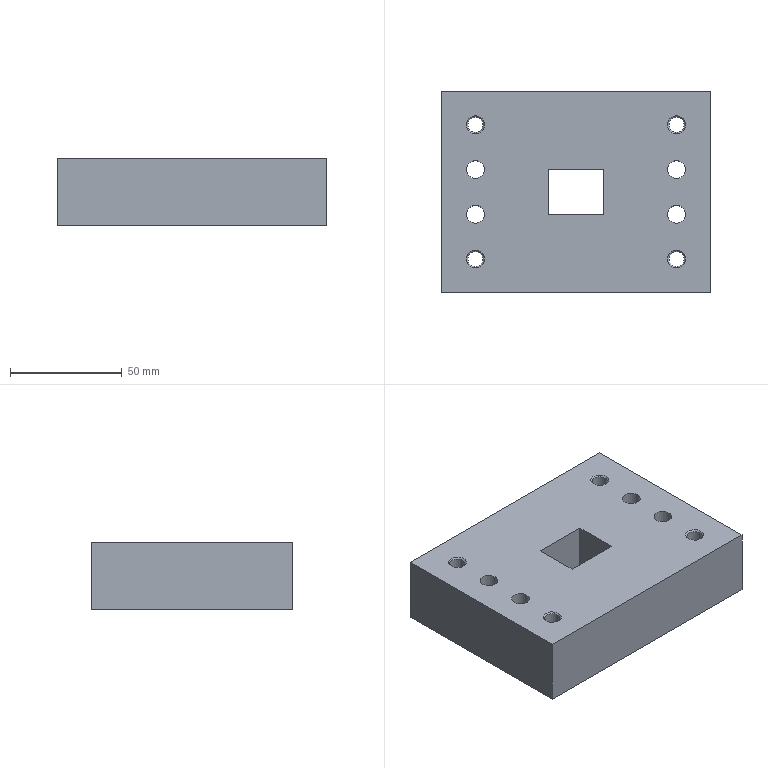Part | NX | features SIMPLE HOLE 4, SYMBOLIC_THREAD 4, DATUM_CSYS 1, EXTRUDE 1, HOLE PACKAGE 1 | 1 solid | 26 faces | box 120 x 90 x 30 mm | volume 298578 mm3 | plane 10 | cylinder 8 | cone 8 | commonest cylinder face diameters 6.8 x4 8 x4
STEP:
#1=CARTESIAN_POINT('',(-12.5,-10.,0.));
#2=VERTEX_POINT('',#1);
#3=CARTESIAN_POINT('',(-12.5,10.,0.));
#4=VERTEX_POINT('',#3);
#5=CARTESIAN_POINT('',(-12.5,-10.,0.));
#6=DIRECTION('',(0.,1.,0.));
#7=VECTOR('',#6,1000.);
#8=LINE('',#5,#7);
#9=EDGE_CURVE('',#2,#4,#8,.T.);
#10=ORIENTED_EDGE('',*,*,#9,.T.);
#11=CARTESIAN_POINT('',(-12.5,10.,30.));
#12=VERTEX_POINT('',#11);
#13=CARTESIAN_POINT('',(-12.5,10.,30.));
#14=DIRECTION('',(0.,0.,-1.));
#15=VECTOR('',#14,1000.);
#16=LINE('',#13,#15);
#17=EDGE_CURVE('',#12,#4,#16,.T.);
#18=ORIENTED_EDGE('',*,*,#17,.F.);
#19=CARTESIAN_POINT('',(-12.5,-10.,30.));
#20=VERTEX_POINT('',#19);
#21=CARTESIAN_POINT('',(-12.5,-10.,30.));
#22=DIRECTION('',(0.,1.,0.));
#23=VECTOR('',#22,1000.);
#24=LINE('',#21,#23);
#25=EDGE_CURVE('',#20,#12,#24,.T.);
#26=ORIENTED_EDGE('',*,*,#25,.F.);
#27=CARTESIAN_POINT('',(-12.5,-10.,30.));
#28=DIRECTION('',(0.,0.,-1.));
#29=VECTOR('',#28,1000.);
#30=LINE('',#27,#29);
#31=EDGE_CURVE('',#20,#2,#30,.T.);
#32=ORIENTED_EDGE('',*,*,#31,.T.);
#33=EDGE_LOOP('',(#10,#18,#26,#32));
#34=FACE_BOUND('',#33,.T.);
#35=CARTESIAN_POINT('',(-12.5,-10.,30.));
#36=DIRECTION('',(-1.,0.,0.));
#37=DIRECTION('',(0.,0.,1.));
#38=AXIS2_PLACEMENT_3D('',#35,#36,#37);
#39=PLANE('',#38);
#40=ADVANCED_FACE('',(#34),#39,.F.);
#41=CARTESIAN_POINT('',(12.5,10.,0.));
#42=VERTEX_POINT('',#41);
#43=CARTESIAN_POINT('',(-12.5,10.,0.));
#44=DIRECTION('',(1.,0.,0.));
#45=VECTOR('',#44,1000.);
#46=LINE('',#43,#45);
#47=EDGE_CURVE('',#4,#42,#46,.T.);
#48=ORIENTED_EDGE('',*,*,#47,.T.);
#49=CARTESIAN_POINT('',(12.5,10.,30.));
#50=VERTEX_POINT('',#49);
#51=CARTESIAN_POINT('',(12.5,10.,30.));
#52=DIRECTION('',(0.,0.,-1.));
#53=VECTOR('',#52,1000.);
#54=LINE('',#51,#53);
#55=EDGE_CURVE('',#50,#42,#54,.T.);
#56=ORIENTED_EDGE('',*,*,#55,.F.);
#57=CARTESIAN_POINT('',(-12.5,10.,30.));
#58=DIRECTION('',(1.,0.,0.));
#59=VECTOR('',#58,1000.);
#60=LINE('',#57,#59);
#61=EDGE_CURVE('',#12,#50,#60,.T.);
#62=ORIENTED_EDGE('',*,*,#61,.F.);
#63=ORIENTED_EDGE('',*,*,#17,.T.);
#64=EDGE_LOOP('',(#48,#56,#62,#63));
#65=FACE_BOUND('',#64,.T.);
#66=CARTESIAN_POINT('',(-12.5,10.,30.));
#67=DIRECTION('',(0.,1.,0.));
#68=DIRECTION('',(0.,0.,1.));
#69=AXIS2_PLACEMENT_3D('',#66,#67,#68);
#70=PLANE('',#69);
#71=ADVANCED_FACE('',(#65),#70,.F.);
#72=CARTESIAN_POINT('',(12.5,-10.,0.));
#73=VERTEX_POINT('',#72);
#74=CARTESIAN_POINT('',(12.5,10.,0.));
#75=DIRECTION('',(0.,-1.,0.));
#76=VECTOR('',#75,1000.);
#77=LINE('',#74,#76);
#78=EDGE_CURVE('',#42,#73,#77,.T.);
#79=ORIENTED_EDGE('',*,*,#78,.T.);
#80=CARTESIAN_POINT('',(12.5,-10.,30.));
#81=VERTEX_POINT('',#80);
#82=CARTESIAN_POINT('',(12.5,-10.,30.));
#83=DIRECTION('',(0.,0.,-1.));
#84=VECTOR('',#83,1000.);
#85=LINE('',#82,#84);
#86=EDGE_CURVE('',#81,#73,#85,.T.);
#87=ORIENTED_EDGE('',*,*,#86,.F.);
#88=CARTESIAN_POINT('',(12.5,10.,30.));
#89=DIRECTION('',(0.,-1.,0.));
#90=VECTOR('',#89,1000.);
#91=LINE('',#88,#90);
#92=EDGE_CURVE('',#50,#81,#91,.T.);
#93=ORIENTED_EDGE('',*,*,#92,.F.);
#94=ORIENTED_EDGE('',*,*,#55,.T.);
#95=EDGE_LOOP('',(#79,#87,#93,#94));
#96=FACE_BOUND('',#95,.T.);
#97=CARTESIAN_POINT('',(12.5,10.,30.));
#98=DIRECTION('',(1.,0.,0.));
#99=DIRECTION('',(0.,0.,-1.));
#100=AXIS2_PLACEMENT_3D('',#97,#98,#99);
#101=PLANE('',#100);
#102=ADVANCED_FACE('',(#96),#101,.F.);
#103=CARTESIAN_POINT('',(-60.,45.,0.));
#104=VERTEX_POINT('',#103);
#105=CARTESIAN_POINT('',(-60.,-45.,0.));
#106=VERTEX_POINT('',#105);
#107=CARTESIAN_POINT('',(-60.,45.,0.));
#108=DIRECTION('',(0.,-1.,0.));
#109=VECTOR('',#108,1000.);
#110=LINE('',#107,#109);
#111=EDGE_CURVE('',#104,#106,#110,.T.);
#112=ORIENTED_EDGE('',*,*,#111,.T.);
#113=CARTESIAN_POINT('',(-60.,-45.,30.));
#114=VERTEX_POINT('',#113);
#115=CARTESIAN_POINT('',(-60.,-45.,30.));
#116=DIRECTION('',(0.,0.,-1.));
#117=VECTOR('',#116,1000.);
#118=LINE('',#115,#117);
#119=EDGE_CURVE('',#114,#106,#118,.T.);
#120=ORIENTED_EDGE('',*,*,#119,.F.);
#121=CARTESIAN_POINT('',(-60.,45.,30.));
#122=VERTEX_POINT('',#121);
#123=CARTESIAN_POINT('',(-60.,45.,30.));
#124=DIRECTION('',(0.,-1.,0.));
#125=VECTOR('',#124,1000.);
#126=LINE('',#123,#125);
#127=EDGE_CURVE('',#122,#114,#126,.T.);
#128=ORIENTED_EDGE('',*,*,#127,.F.);
#129=CARTESIAN_POINT('',(-60.,45.,30.));
#130=DIRECTION('',(0.,0.,-1.));
#131=VECTOR('',#130,1000.);
#132=LINE('',#129,#131);
#133=EDGE_CURVE('',#122,#104,#132,.T.);
#134=ORIENTED_EDGE('',*,*,#133,.T.);
#135=EDGE_LOOP('',(#112,#120,#128,#134));
#136=FACE_BOUND('',#135,.T.);
#137=CARTESIAN_POINT('',(-60.,45.,30.));
#138=DIRECTION('',(1.,0.,0.));
#139=DIRECTION('',(0.,0.,-1.));
#140=AXIS2_PLACEMENT_3D('',#137,#138,#139);
#141=PLANE('',#140);
#142=ADVANCED_FACE('',(#136),#141,.F.);
#143=CARTESIAN_POINT('',(60.,-45.,0.));
#144=VERTEX_POINT('',#143);
#145=CARTESIAN_POINT('',(-60.,-45.,0.));
#146=DIRECTION('',(1.,0.,0.));
#147=VECTOR('',#146,1000.);
#148=LINE('',#145,#147);
#149=EDGE_CURVE('',#106,#144,#148,.T.);
#150=ORIENTED_EDGE('',*,*,#149,.T.);
#151=CARTESIAN_POINT('',(60.,-45.,30.));
#152=VERTEX_POINT('',#151);
#153=CARTESIAN_POINT('',(60.,-45.,30.));
#154=DIRECTION('',(0.,0.,-1.));
#155=VECTOR('',#154,1000.);
#156=LINE('',#153,#155);
#157=EDGE_CURVE('',#152,#144,#156,.T.);
#158=ORIENTED_EDGE('',*,*,#157,.F.);
#159=CARTESIAN_POINT('',(-60.,-45.,30.));
#160=DIRECTION('',(1.,0.,0.));
#161=VECTOR('',#160,1000.);
#162=LINE('',#159,#161);
#163=EDGE_CURVE('',#114,#152,#162,.T.);
#164=ORIENTED_EDGE('',*,*,#163,.F.);
#165=ORIENTED_EDGE('',*,*,#119,.T.);
#166=EDGE_LOOP('',(#150,#158,#164,#165));
#167=FACE_BOUND('',#166,.T.);
#168=CARTESIAN_POINT('',(-60.,-45.,30.));
#169=DIRECTION('',(0.,1.,0.));
#170=DIRECTION('',(0.,0.,1.));
#171=AXIS2_PLACEMENT_3D('',#168,#169,#170);
#172=PLANE('',#171);
#173=ADVANCED_FACE('',(#167),#172,.F.);
#174=CARTESIAN_POINT('',(60.,45.,0.));
#175=VERTEX_POINT('',#174);
#176=CARTESIAN_POINT('',(60.,-45.,0.));
#177=DIRECTION('',(0.,1.,0.));
#178=VECTOR('',#177,1000.);
#179=LINE('',#176,#178);
#180=EDGE_CURVE('',#144,#175,#179,.T.);
#181=ORIENTED_EDGE('',*,*,#180,.T.);
#182=CARTESIAN_POINT('',(60.,45.,30.));
#183=VERTEX_POINT('',#182);
#184=CARTESIAN_POINT('',(60.,45.,30.));
#185=DIRECTION('',(0.,0.,-1.));
#186=VECTOR('',#185,1000.);
#187=LINE('',#184,#186);
#188=EDGE_CURVE('',#183,#175,#187,.T.);
#189=ORIENTED_EDGE('',*,*,#188,.F.);
#190=CARTESIAN_POINT('',(60.,-45.,30.));
#191=DIRECTION('',(0.,1.,0.));
#192=VECTOR('',#191,1000.);
#193=LINE('',#190,#192);
#194=EDGE_CURVE('',#152,#183,#193,.T.);
#195=ORIENTED_EDGE('',*,*,#194,.F.);
#196=ORIENTED_EDGE('',*,*,#157,.T.);
#197=EDGE_LOOP('',(#181,#189,#195,#196));
#198=FACE_BOUND('',#197,.T.);
#199=CARTESIAN_POINT('',(60.,-45.,30.));
#200=DIRECTION('',(-1.,0.,0.));
#201=DIRECTION('',(0.,0.,1.));
#202=AXIS2_PLACEMENT_3D('',#199,#200,#201);
#203=PLANE('',#202);
#204=ADVANCED_FACE('',(#198),#203,.F.);
#205=CARTESIAN_POINT('',(-41.,-10.,30.));
#206=VERTEX_POINT('',#205);
#207=CARTESIAN_POINT('',(-45.,-10.,30.));
#208=DIRECTION('',(0.,0.,1.));
#209=DIRECTION('',(1.,0.,0.));
#210=AXIS2_PLACEMENT_3D('',#207,#208,#209);
#211=CIRCLE('',#210,4.);
#212=EDGE_CURVE('',#206,#206,#211,.T.);
#213=ORIENTED_EDGE('',*,*,#212,.T.);
#214=EDGE_LOOP('',(#213));
#215=FACE_BOUND('',#214,.T.);
#216=CARTESIAN_POINT('',(-41.,-10.,0.));
#217=VERTEX_POINT('',#216);
#218=CARTESIAN_POINT('',(-45.,-10.,0.));
#219=DIRECTION('',(0.,0.,1.));
#220=DIRECTION('',(1.,0.,0.));
#221=AXIS2_PLACEMENT_3D('',#218,#219,#220);
#222=CIRCLE('',#221,4.);
#223=EDGE_CURVE('',#217,#217,#222,.T.);
#224=ORIENTED_EDGE('',*,*,#223,.F.);
#225=EDGE_LOOP('',(#224));
#226=FACE_BOUND('',#225,.T.);
#227=CARTESIAN_POINT('',(-45.,-10.,30.));
#228=DIRECTION('',(0.,0.,-1.));
#229=DIRECTION('',(-1.,0.,0.));
#230=AXIS2_PLACEMENT_3D('',#227,#228,#229);
#231=CYLINDRICAL_SURFACE('',#230,4.);
#232=ADVANCED_FACE('',(#215,#226),#231,.F.);
#233=CARTESIAN_POINT('',(-41.,10.,30.));
#234=VERTEX_POINT('',#233);
#235=CARTESIAN_POINT('',(-45.,10.,30.));
#236=DIRECTION('',(0.,0.,1.));
#237=DIRECTION('',(1.,0.,0.));
#238=AXIS2_PLACEMENT_3D('',#235,#236,#237);
#239=CIRCLE('',#238,4.);
#240=EDGE_CURVE('',#234,#234,#239,.T.);
#241=ORIENTED_EDGE('',*,*,#240,.T.);
#242=EDGE_LOOP('',(#241));
#243=FACE_BOUND('',#242,.T.);
#244=CARTESIAN_POINT('',(-41.,10.,0.));
#245=VERTEX_POINT('',#244);
#246=CARTESIAN_POINT('',(-45.,10.,0.));
#247=DIRECTION('',(0.,0.,1.));
#248=DIRECTION('',(1.,0.,0.));
#249=AXIS2_PLACEMENT_3D('',#246,#247,#248);
#250=CIRCLE('',#249,4.);
#251=EDGE_CURVE('',#245,#245,#250,.T.);
#252=ORIENTED_EDGE('',*,*,#251,.F.);
#253=EDGE_LOOP('',(#252));
#254=FACE_BOUND('',#253,.T.);
#255=CARTESIAN_POINT('',(-45.,10.,30.));
#256=DIRECTION('',(0.,0.,-1.));
#257=DIRECTION('',(-1.,0.,0.));
#258=AXIS2_PLACEMENT_3D('',#255,#256,#257);
#259=CYLINDRICAL_SURFACE('',#258,4.);
#260=ADVANCED_FACE('',(#243,#254),#259,.F.);
#261=CARTESIAN_POINT('',(49.,-10.,30.));
#262=VERTEX_POINT('',#261);
#263=CARTESIAN_POINT('',(45.,-10.,30.));
#264=DIRECTION('',(0.,0.,1.));
#265=DIRECTION('',(1.,0.,0.));
#266=AXIS2_PLACEMENT_3D('',#263,#264,#265);
#267=CIRCLE('',#266,4.);
#268=EDGE_CURVE('',#262,#262,#267,.T.);
#269=ORIENTED_EDGE('',*,*,#268,.T.);
#270=EDGE_LOOP('',(#269));
#271=FACE_BOUND('',#270,.T.);
#272=CARTESIAN_POINT('',(49.,-10.,0.));
#273=VERTEX_POINT('',#272);
#274=CARTESIAN_POINT('',(45.,-10.,0.));
#275=DIRECTION('',(0.,0.,1.));
#276=DIRECTION('',(1.,0.,0.));
#277=AXIS2_PLACEMENT_3D('',#274,#275,#276);
#278=CIRCLE('',#277,4.);
#279=EDGE_CURVE('',#273,#273,#278,.T.);
#280=ORIENTED_EDGE('',*,*,#279,.F.);
#281=EDGE_LOOP('',(#280));
#282=FACE_BOUND('',#281,.T.);
#283=CARTESIAN_POINT('',(45.,-10.,30.));
#284=DIRECTION('',(0.,0.,-1.));
#285=DIRECTION('',(-1.,0.,0.));
#286=AXIS2_PLACEMENT_3D('',#283,#284,#285);
#287=CYLINDRICAL_SURFACE('',#286,4.);
#288=ADVANCED_FACE('',(#271,#282),#287,.F.);
#289=CARTESIAN_POINT('',(49.,10.,30.));
#290=VERTEX_POINT('',#289);
#291=CARTESIAN_POINT('',(45.,10.,30.));
#292=DIRECTION('',(0.,0.,1.));
#293=DIRECTION('',(1.,0.,0.));
#294=AXIS2_PLACEMENT_3D('',#291,#292,#293);
#295=CIRCLE('',#294,4.);
#296=EDGE_CURVE('',#290,#290,#295,.T.);
#297=ORIENTED_EDGE('',*,*,#296,.T.);
#298=EDGE_LOOP('',(#297));
#299=FACE_BOUND('',#298,.T.);
#300=CARTESIAN_POINT('',(49.,10.,0.));
#301=VERTEX_POINT('',#300);
#302=CARTESIAN_POINT('',(45.,10.,0.));
#303=DIRECTION('',(0.,0.,1.));
#304=DIRECTION('',(1.,0.,0.));
#305=AXIS2_PLACEMENT_3D('',#302,#303,#304);
#306=CIRCLE('',#305,4.);
#307=EDGE_CURVE('',#301,#301,#306,.T.);
#308=ORIENTED_EDGE('',*,*,#307,.F.);
#309=EDGE_LOOP('',(#308));
#310=FACE_BOUND('',#309,.T.);
#311=CARTESIAN_POINT('',(45.,10.,30.));
#312=DIRECTION('',(0.,0.,-1.));
#313=DIRECTION('',(-1.,0.,0.));
#314=AXIS2_PLACEMENT_3D('',#311,#312,#313);
#315=CYLINDRICAL_SURFACE('',#314,4.);
#316=ADVANCED_FACE('',(#299,#310),#315,.F.);
#317=CARTESIAN_POINT('',(60.,45.,0.));
#318=DIRECTION('',(-1.,0.,0.));
#319=VECTOR('',#318,1000.);
#320=LINE('',#317,#319);
#321=EDGE_CURVE('',#175,#104,#320,.T.);
#322=ORIENTED_EDGE('',*,*,#321,.T.);
#323=ORIENTED_EDGE('',*,*,#133,.F.);
#324=CARTESIAN_POINT('',(60.,45.,30.));
#325=DIRECTION('',(-1.,0.,0.));
#326=VECTOR('',#325,1000.);
#327=LINE('',#324,#326);
#328=EDGE_CURVE('',#183,#122,#327,.T.);
#329=ORIENTED_EDGE('',*,*,#328,.F.);
#330=ORIENTED_EDGE('',*,*,#188,.T.);
#331=EDGE_LOOP('',(#322,#323,#329,#330));
#332=FACE_BOUND('',#331,.T.);
#333=CARTESIAN_POINT('',(60.,45.,30.));
#334=DIRECTION('',(0.,-1.,0.));
#335=DIRECTION('',(0.,0.,-1.));
#336=AXIS2_PLACEMENT_3D('',#333,#334,#335);
#337=PLANE('',#336);
#338=ADVANCED_FACE('',(#332),#337,.F.);
#339=CARTESIAN_POINT('',(12.5,-10.,0.));
#340=DIRECTION('',(-1.,0.,0.));
#341=VECTOR('',#340,1000.);
#342=LINE('',#339,#341);
#343=EDGE_CURVE('',#73,#2,#342,.T.);
#344=ORIENTED_EDGE('',*,*,#343,.T.);
#345=ORIENTED_EDGE('',*,*,#31,.F.);
#346=CARTESIAN_POINT('',(12.5,-10.,30.));
#347=DIRECTION('',(-1.,0.,0.));
#348=VECTOR('',#347,1000.);
#349=LINE('',#346,#348);
#350=EDGE_CURVE('',#81,#20,#349,.T.);
#351=ORIENTED_EDGE('',*,*,#350,.F.);
#352=ORIENTED_EDGE('',*,*,#86,.T.);
#353=EDGE_LOOP('',(#344,#345,#351,#352));
#354=FACE_BOUND('',#353,.T.);
#355=CARTESIAN_POINT('',(12.5,-10.,30.));
#356=DIRECTION('',(0.,-1.,0.));
#357=DIRECTION('',(0.,0.,-1.));
#358=AXIS2_PLACEMENT_3D('',#355,#356,#357);
#359=PLANE('',#358);
#360=ADVANCED_FACE('',(#354),#359,.F.);
#361=CARTESIAN_POINT('',(49.,-30.,30.));
#362=VERTEX_POINT('',#361);
#363=CARTESIAN_POINT('',(45.,-30.,30.));
#364=DIRECTION('',(0.,0.,1.));
#365=DIRECTION('',(1.,0.,0.));
#366=AXIS2_PLACEMENT_3D('',#363,#364,#365);
#367=CIRCLE('',#366,4.);
#368=EDGE_CURVE('',#362,#362,#367,.F.);
#369=ORIENTED_EDGE('',*,*,#368,.T.);
#370=EDGE_LOOP('',(#369));
#371=FACE_BOUND('',#370,.T.);
#372=CARTESIAN_POINT('',(49.,30.,30.));
#373=VERTEX_POINT('',#372);
#374=CARTESIAN_POINT('',(45.,30.,30.));
#375=DIRECTION('',(0.,0.,1.));
#376=DIRECTION('',(1.,0.,0.));
#377=AXIS2_PLACEMENT_3D('',#374,#375,#376);
#378=CIRCLE('',#377,4.);
#379=EDGE_CURVE('',#373,#373,#378,.F.);
#380=ORIENTED_EDGE('',*,*,#379,.T.);
#381=EDGE_LOOP('',(#380));
#382=FACE_BOUND('',#381,.T.);
#383=CARTESIAN_POINT('',(-41.,30.,30.));
#384=VERTEX_POINT('',#383);
#385=CARTESIAN_POINT('',(-45.,30.,30.));
#386=DIRECTION('',(0.,0.,1.));
#387=DIRECTION('',(1.,0.,0.));
#388=AXIS2_PLACEMENT_3D('',#385,#386,#387);
#389=CIRCLE('',#388,4.);
#390=EDGE_CURVE('',#384,#384,#389,.F.);
#391=ORIENTED_EDGE('',*,*,#390,.T.);
#392=EDGE_LOOP('',(#391));
#393=FACE_BOUND('',#392,.T.);
#394=CARTESIAN_POINT('',(-41.,-30.,30.));
#395=VERTEX_POINT('',#394);
#396=CARTESIAN_POINT('',(-45.,-30.,30.));
#397=DIRECTION('',(0.,0.,1.));
#398=DIRECTION('',(1.,0.,0.));
#399=AXIS2_PLACEMENT_3D('',#396,#397,#398);
#400=CIRCLE('',#399,4.);
#401=EDGE_CURVE('',#395,#395,#400,.F.);
#402=ORIENTED_EDGE('',*,*,#401,.T.);
#403=EDGE_LOOP('',(#402));
#404=FACE_BOUND('',#403,.T.);
#405=ORIENTED_EDGE('',*,*,#127,.T.);
#406=ORIENTED_EDGE('',*,*,#163,.T.);
#407=ORIENTED_EDGE('',*,*,#194,.T.);
#408=ORIENTED_EDGE('',*,*,#328,.T.);
#409=EDGE_LOOP('',(#405,#406,#407,#408));
#410=FACE_BOUND('',#409,.T.);
#411=ORIENTED_EDGE('',*,*,#296,.F.);
#412=EDGE_LOOP('',(#411));
#413=FACE_BOUND('',#412,.T.);
#414=ORIENTED_EDGE('',*,*,#268,.F.);
#415=EDGE_LOOP('',(#414));
#416=FACE_BOUND('',#415,.T.);
#417=ORIENTED_EDGE('',*,*,#240,.F.);
#418=EDGE_LOOP('',(#417));
#419=FACE_BOUND('',#418,.T.);
#420=ORIENTED_EDGE('',*,*,#212,.F.);
#421=EDGE_LOOP('',(#420));
#422=FACE_BOUND('',#421,.T.);
#423=ORIENTED_EDGE('',*,*,#25,.T.);
#424=ORIENTED_EDGE('',*,*,#61,.T.);
#425=ORIENTED_EDGE('',*,*,#92,.T.);
#426=ORIENTED_EDGE('',*,*,#350,.T.);
#427=EDGE_LOOP('',(#423,#424,#425,#426));
#428=FACE_BOUND('',#427,.T.);
#429=CARTESIAN_POINT('',(45.,10.,30.));
#430=DIRECTION('',(0.,0.,1.));
#431=DIRECTION('',(1.,0.,0.));
#432=AXIS2_PLACEMENT_3D('',#429,#430,#431);
#433=PLANE('',#432);
#434=ADVANCED_FACE('',(#371,#382,#393,#404,#410,#413,#416,#419,#422,#428),#433,.T.);
#435=CARTESIAN_POINT('',(49.,-30.,0.));
#436=VERTEX_POINT('',#435);
#437=CARTESIAN_POINT('',(45.,-30.,0.));
#438=DIRECTION('',(0.,0.,1.));
#439=DIRECTION('',(1.,0.,0.));
#440=AXIS2_PLACEMENT_3D('',#437,#438,#439);
#441=CIRCLE('',#440,4.);
#442=EDGE_CURVE('',#436,#436,#441,.T.);
#443=ORIENTED_EDGE('',*,*,#442,.T.);
#444=EDGE_LOOP('',(#443));
#445=FACE_BOUND('',#444,.T.);
#446=CARTESIAN_POINT('',(49.,30.,0.));
#447=VERTEX_POINT('',#446);
#448=CARTESIAN_POINT('',(45.,30.,0.));
#449=DIRECTION('',(0.,0.,1.));
#450=DIRECTION('',(1.,0.,0.));
#451=AXIS2_PLACEMENT_3D('',#448,#449,#450);
#452=CIRCLE('',#451,4.);
#453=EDGE_CURVE('',#447,#447,#452,.T.);
#454=ORIENTED_EDGE('',*,*,#453,.T.);
#455=EDGE_LOOP('',(#454));
#456=FACE_BOUND('',#455,.T.);
#457=CARTESIAN_POINT('',(-41.,30.,0.));
#458=VERTEX_POINT('',#457);
#459=CARTESIAN_POINT('',(-45.,30.,0.));
#460=DIRECTION('',(0.,0.,1.));
#461=DIRECTION('',(1.,0.,0.));
#462=AXIS2_PLACEMENT_3D('',#459,#460,#461);
#463=CIRCLE('',#462,4.);
#464=EDGE_CURVE('',#458,#458,#463,.T.);
#465=ORIENTED_EDGE('',*,*,#464,.T.);
#466=EDGE_LOOP('',(#465));
#467=FACE_BOUND('',#466,.T.);
#468=CARTESIAN_POINT('',(-41.,-30.,0.));
#469=VERTEX_POINT('',#468);
#470=CARTESIAN_POINT('',(-45.,-30.,0.));
#471=DIRECTION('',(0.,0.,1.));
#472=DIRECTION('',(1.,0.,0.));
#473=AXIS2_PLACEMENT_3D('',#470,#471,#472);
#474=CIRCLE('',#473,4.);
#475=EDGE_CURVE('',#469,#469,#474,.T.);
#476=ORIENTED_EDGE('',*,*,#475,.T.);
#477=EDGE_LOOP('',(#476));
#478=FACE_BOUND('',#477,.T.);
#479=ORIENTED_EDGE('',*,*,#111,.F.);
#480=ORIENTED_EDGE('',*,*,#321,.F.);
#481=ORIENTED_EDGE('',*,*,#180,.F.);
#482=ORIENTED_EDGE('',*,*,#149,.F.);
#483=EDGE_LOOP('',(#479,#480,#481,#482));
#484=FACE_BOUND('',#483,.T.);
#485=ORIENTED_EDGE('',*,*,#307,.T.);
#486=EDGE_LOOP('',(#485));
#487=FACE_BOUND('',#486,.T.);
#488=ORIENTED_EDGE('',*,*,#279,.T.);
#489=EDGE_LOOP('',(#488));
#490=FACE_BOUND('',#489,.T.);
#491=ORIENTED_EDGE('',*,*,#251,.T.);
#492=EDGE_LOOP('',(#491));
#493=FACE_BOUND('',#492,.T.);
#494=ORIENTED_EDGE('',*,*,#223,.T.);
#495=EDGE_LOOP('',(#494));
#496=FACE_BOUND('',#495,.T.);
#497=ORIENTED_EDGE('',*,*,#9,.F.);
#498=ORIENTED_EDGE('',*,*,#343,.F.);
#499=ORIENTED_EDGE('',*,*,#78,.F.);
#500=ORIENTED_EDGE('',*,*,#47,.F.);
#501=EDGE_LOOP('',(#497,#498,#499,#500));
#502=FACE_BOUND('',#501,.T.);
#503=CARTESIAN_POINT('',(45.,10.,0.));
#504=DIRECTION('',(0.,0.,1.));
#505=DIRECTION('',(1.,0.,0.));
#506=AXIS2_PLACEMENT_3D('',#503,#504,#505);
#507=PLANE('',#506);
#508=ADVANCED_FACE('',(#445,#456,#467,#478,#484,#487,#490,#493,#496,#502),#507,.F.);
#509=CARTESIAN_POINT('',(-41.6,-30.,29.4));
#510=VERTEX_POINT('',#509);
#511=CARTESIAN_POINT('',(-45.,-30.,29.4));
#512=DIRECTION('',(0.,0.,1.));
#513=DIRECTION('',(1.,0.,0.));
#514=AXIS2_PLACEMENT_3D('',#511,#512,#513);
#515=CIRCLE('',#514,3.4);
#516=EDGE_CURVE('',#510,#510,#515,.T.);
#517=ORIENTED_EDGE('',*,*,#516,.T.);
#518=EDGE_LOOP('',(#517));
#519=FACE_BOUND('',#518,.T.);
#520=CARTESIAN_POINT('',(-41.6,-30.,0.6));
#521=VERTEX_POINT('',#520);
#522=CARTESIAN_POINT('',(-45.,-30.,0.6));
#523=DIRECTION('',(0.,0.,1.));
#524=DIRECTION('',(1.,0.,0.));
#525=AXIS2_PLACEMENT_3D('',#522,#523,#524);
#526=CIRCLE('',#525,3.4);
#527=EDGE_CURVE('',#521,#521,#526,.F.);
#528=ORIENTED_EDGE('',*,*,#527,.T.);
#529=EDGE_LOOP('',(#528));
#530=FACE_BOUND('',#529,.T.);
#531=CARTESIAN_POINT('',(-45.,-30.,0.));
#532=DIRECTION('',(0.,0.,1.));
#533=DIRECTION('',(1.,0.,0.));
#534=AXIS2_PLACEMENT_3D('',#531,#532,#533);
#535=CYLINDRICAL_SURFACE('',#534,3.4);
#536=ADVANCED_FACE('',(#519,#530),#535,.F.);
#537=ORIENTED_EDGE('',*,*,#527,.F.);
#538=EDGE_LOOP('',(#537));
#539=FACE_BOUND('',#538,.T.);
#540=ORIENTED_EDGE('',*,*,#475,.F.);
#541=EDGE_LOOP('',(#540));
#542=FACE_BOUND('',#541,.T.);
#543=CARTESIAN_POINT('',(-45.,-30.,0.));
#544=DIRECTION('',(0.,0.,-1.));
#545=DIRECTION('',(-1.,0.,0.));
#546=AXIS2_PLACEMENT_3D('',#543,#544,#545);
#547=CONICAL_SURFACE('',#546,4.,0.7854);
#548=ADVANCED_FACE('',(#539,#542),#547,.F.);
#549=ORIENTED_EDGE('',*,*,#401,.F.);
#550=EDGE_LOOP('',(#549));
#551=FACE_BOUND('',#550,.T.);
#552=ORIENTED_EDGE('',*,*,#516,.F.);
#553=EDGE_LOOP('',(#552));
#554=FACE_BOUND('',#553,.T.);
#555=CARTESIAN_POINT('',(-45.,-30.,29.4));
#556=DIRECTION('',(0.,0.,1.));
#557=DIRECTION('',(1.,0.,0.));
#558=AXIS2_PLACEMENT_3D('',#555,#556,#557);
#559=CONICAL_SURFACE('',#558,3.4,0.7854);
#560=ADVANCED_FACE('',(#551,#554),#559,.F.);
#561=CARTESIAN_POINT('',(-41.6,30.,29.4));
#562=VERTEX_POINT('',#561);
#563=CARTESIAN_POINT('',(-45.,30.,29.4));
#564=DIRECTION('',(0.,0.,1.));
#565=DIRECTION('',(1.,0.,0.));
#566=AXIS2_PLACEMENT_3D('',#563,#564,#565);
#567=CIRCLE('',#566,3.4);
#568=EDGE_CURVE('',#562,#562,#567,.T.);
#569=ORIENTED_EDGE('',*,*,#568,.T.);
#570=EDGE_LOOP('',(#569));
#571=FACE_BOUND('',#570,.T.);
#572=CARTESIAN_POINT('',(-41.6,30.,0.6));
#573=VERTEX_POINT('',#572);
#574=CARTESIAN_POINT('',(-45.,30.,0.6));
#575=DIRECTION('',(0.,0.,1.));
#576=DIRECTION('',(1.,0.,0.));
#577=AXIS2_PLACEMENT_3D('',#574,#575,#576);
#578=CIRCLE('',#577,3.4);
#579=EDGE_CURVE('',#573,#573,#578,.F.);
#580=ORIENTED_EDGE('',*,*,#579,.T.);
#581=EDGE_LOOP('',(#580));
#582=FACE_BOUND('',#581,.T.);
#583=CARTESIAN_POINT('',(-45.,30.,0.));
#584=DIRECTION('',(0.,0.,1.));
#585=DIRECTION('',(1.,0.,0.));
#586=AXIS2_PLACEMENT_3D('',#583,#584,#585);
#587=CYLINDRICAL_SURFACE('',#586,3.4);
#588=ADVANCED_FACE('',(#571,#582),#587,.F.);
#589=ORIENTED_EDGE('',*,*,#579,.F.);
#590=EDGE_LOOP('',(#589));
#591=FACE_BOUND('',#590,.T.);
#592=ORIENTED_EDGE('',*,*,#464,.F.);
#593=EDGE_LOOP('',(#592));
#594=FACE_BOUND('',#593,.T.);
#595=CARTESIAN_POINT('',(-45.,30.,0.));
#596=DIRECTION('',(0.,0.,-1.));
#597=DIRECTION('',(-1.,0.,0.));
#598=AXIS2_PLACEMENT_3D('',#595,#596,#597);
#599=CONICAL_SURFACE('',#598,4.,0.7854);
#600=ADVANCED_FACE('',(#591,#594),#599,.F.);
#601=ORIENTED_EDGE('',*,*,#390,.F.);
#602=EDGE_LOOP('',(#601));
#603=FACE_BOUND('',#602,.T.);
#604=ORIENTED_EDGE('',*,*,#568,.F.);
#605=EDGE_LOOP('',(#604));
#606=FACE_BOUND('',#605,.T.);
#607=CARTESIAN_POINT('',(-45.,30.,29.4));
#608=DIRECTION('',(0.,0.,1.));
#609=DIRECTION('',(1.,0.,0.));
#610=AXIS2_PLACEMENT_3D('',#607,#608,#609);
#611=CONICAL_SURFACE('',#610,3.4,0.7854);
#612=ADVANCED_FACE('',(#603,#606),#611,.F.);
#613=CARTESIAN_POINT('',(48.4,30.,29.4));
#614=VERTEX_POINT('',#613);
#615=CARTESIAN_POINT('',(45.,30.,29.4));
#616=DIRECTION('',(0.,0.,1.));
#617=DIRECTION('',(1.,0.,0.));
#618=AXIS2_PLACEMENT_3D('',#615,#616,#617);
#619=CIRCLE('',#618,3.4);
#620=EDGE_CURVE('',#614,#614,#619,.T.);
#621=ORIENTED_EDGE('',*,*,#620,.T.);
#622=EDGE_LOOP('',(#621));
#623=FACE_BOUND('',#622,.T.);
#624=CARTESIAN_POINT('',(48.4,30.,0.6));
#625=VERTEX_POINT('',#624);
#626=CARTESIAN_POINT('',(45.,30.,0.6));
#627=DIRECTION('',(0.,0.,1.));
#628=DIRECTION('',(1.,0.,0.));
#629=AXIS2_PLACEMENT_3D('',#626,#627,#628);
#630=CIRCLE('',#629,3.4);
#631=EDGE_CURVE('',#625,#625,#630,.F.);
#632=ORIENTED_EDGE('',*,*,#631,.T.);
#633=EDGE_LOOP('',(#632));
#634=FACE_BOUND('',#633,.T.);
#635=CARTESIAN_POINT('',(45.,30.,0.));
#636=DIRECTION('',(0.,0.,1.));
#637=DIRECTION('',(1.,0.,0.));
#638=AXIS2_PLACEMENT_3D('',#635,#636,#637);
#639=CYLINDRICAL_SURFACE('',#638,3.4);
#640=ADVANCED_FACE('',(#623,#634),#639,.F.);
#641=ORIENTED_EDGE('',*,*,#631,.F.);
#642=EDGE_LOOP('',(#641));
#643=FACE_BOUND('',#642,.T.);
#644=ORIENTED_EDGE('',*,*,#453,.F.);
#645=EDGE_LOOP('',(#644));
#646=FACE_BOUND('',#645,.T.);
#647=CARTESIAN_POINT('',(45.,30.,0.));
#648=DIRECTION('',(0.,0.,-1.));
#649=DIRECTION('',(-1.,0.,0.));
#650=AXIS2_PLACEMENT_3D('',#647,#648,#649);
#651=CONICAL_SURFACE('',#650,4.,0.7854);
#652=ADVANCED_FACE('',(#643,#646),#651,.F.);
#653=ORIENTED_EDGE('',*,*,#379,.F.);
#654=EDGE_LOOP('',(#653));
#655=FACE_BOUND('',#654,.T.);
#656=ORIENTED_EDGE('',*,*,#620,.F.);
#657=EDGE_LOOP('',(#656));
#658=FACE_BOUND('',#657,.T.);
#659=CARTESIAN_POINT('',(45.,30.,29.4));
#660=DIRECTION('',(0.,0.,1.));
#661=DIRECTION('',(1.,0.,0.));
#662=AXIS2_PLACEMENT_3D('',#659,#660,#661);
#663=CONICAL_SURFACE('',#662,3.4,0.7854);
#664=ADVANCED_FACE('',(#655,#658),#663,.F.);
#665=CARTESIAN_POINT('',(48.4,-30.,29.4));
#666=VERTEX_POINT('',#665);
#667=CARTESIAN_POINT('',(45.,-30.,29.4));
#668=DIRECTION('',(0.,0.,1.));
#669=DIRECTION('',(1.,0.,0.));
#670=AXIS2_PLACEMENT_3D('',#667,#668,#669);
#671=CIRCLE('',#670,3.4);
#672=EDGE_CURVE('',#666,#666,#671,.T.);
#673=ORIENTED_EDGE('',*,*,#672,.T.);
#674=EDGE_LOOP('',(#673));
#675=FACE_BOUND('',#674,.T.);
#676=CARTESIAN_POINT('',(48.4,-30.,0.6));
#677=VERTEX_POINT('',#676);
#678=CARTESIAN_POINT('',(45.,-30.,0.6));
#679=DIRECTION('',(0.,0.,1.));
#680=DIRECTION('',(1.,0.,0.));
#681=AXIS2_PLACEMENT_3D('',#678,#679,#680);
#682=CIRCLE('',#681,3.4);
#683=EDGE_CURVE('',#677,#677,#682,.F.);
#684=ORIENTED_EDGE('',*,*,#683,.T.);
#685=EDGE_LOOP('',(#684));
#686=FACE_BOUND('',#685,.T.);
#687=CARTESIAN_POINT('',(45.,-30.,0.));
#688=DIRECTION('',(0.,0.,1.));
#689=DIRECTION('',(1.,0.,0.));
#690=AXIS2_PLACEMENT_3D('',#687,#688,#689);
#691=CYLINDRICAL_SURFACE('',#690,3.4);
#692=ADVANCED_FACE('',(#675,#686),#691,.F.);
#693=ORIENTED_EDGE('',*,*,#683,.F.);
#694=EDGE_LOOP('',(#693));
#695=FACE_BOUND('',#694,.T.);
#696=ORIENTED_EDGE('',*,*,#442,.F.);
#697=EDGE_LOOP('',(#696));
#698=FACE_BOUND('',#697,.T.);
#699=CARTESIAN_POINT('',(45.,-30.,0.));
#700=DIRECTION('',(0.,0.,-1.));
#701=DIRECTION('',(-1.,0.,0.));
#702=AXIS2_PLACEMENT_3D('',#699,#700,#701);
#703=CONICAL_SURFACE('',#702,4.,0.7854);
#704=ADVANCED_FACE('',(#695,#698),#703,.F.);
#705=ORIENTED_EDGE('',*,*,#368,.F.);
#706=EDGE_LOOP('',(#705));
#707=FACE_BOUND('',#706,.T.);
#708=ORIENTED_EDGE('',*,*,#672,.F.);
#709=EDGE_LOOP('',(#708));
#710=FACE_BOUND('',#709,.T.);
#711=CARTESIAN_POINT('',(45.,-30.,29.4));
#712=DIRECTION('',(0.,0.,1.));
#713=DIRECTION('',(1.,0.,0.));
#714=AXIS2_PLACEMENT_3D('',#711,#712,#713);
#715=CONICAL_SURFACE('',#714,3.4,0.7854);
#716=ADVANCED_FACE('',(#707,#710),#715,.F.);
#717=CLOSED_SHELL('',(#40,#71,#102,#142,#173,#204,#232,#260,#288,#316,#338,#360,#434,#508,#536,#548,#560,#588,#600,#612,#640,#652,#664,#692,#704,#716));
#718=MANIFOLD_SOLID_BREP('',#717);
#719=(LENGTH_UNIT()NAMED_UNIT(*)SI_UNIT(.MILLI.,.METRE.));
#720=UNCERTAINTY_MEASURE_WITH_UNIT(LENGTH_MEASURE(0.00001),#719,'','');
#721=(NAMED_UNIT(*)PLANE_ANGLE_UNIT()SI_UNIT($,.RADIAN.));
#722=(NAMED_UNIT(*)SI_UNIT($,.STERADIAN.)SOLID_ANGLE_UNIT());
#723=(GEOMETRIC_REPRESENTATION_CONTEXT(3)GLOBAL_UNCERTAINTY_ASSIGNED_CONTEXT((#720))GLOBAL_UNIT_ASSIGNED_CONTEXT((#719,#721,#722))REPRESENTATION_CONTEXT('',''));
#724=ADVANCED_BREP_SHAPE_REPRESENTATION('',(#718),#723);